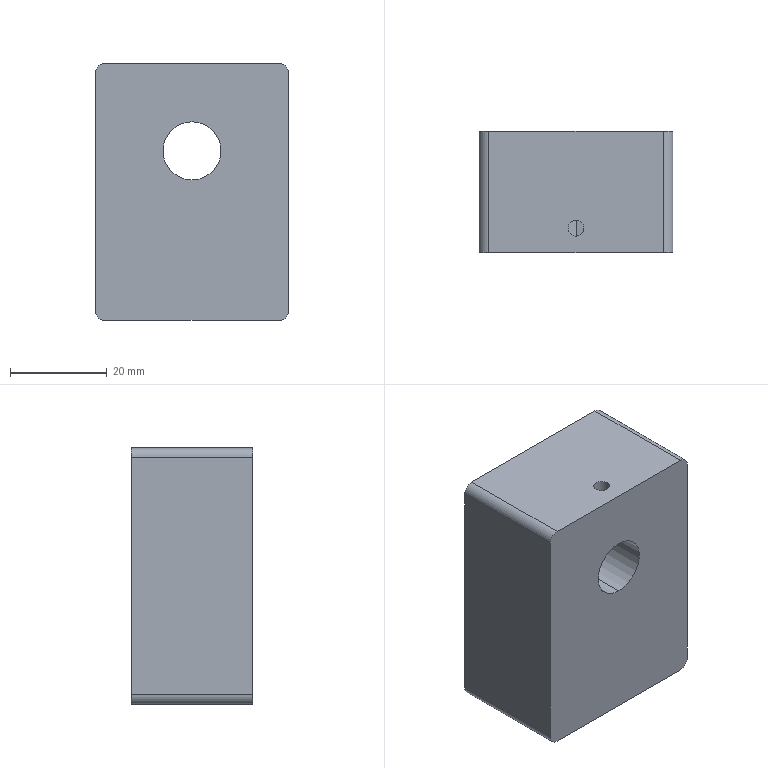Part | STEP file | 1 solid | 53 faces | box 40 x 25 x 53 mm | volume 43545 mm3 | cylinder 28 | cone 18 | plane 7 | commonest cylinder face diameters 5 x8 2.5 x6 4 x4 8 x4 3.3 x2 12 x2